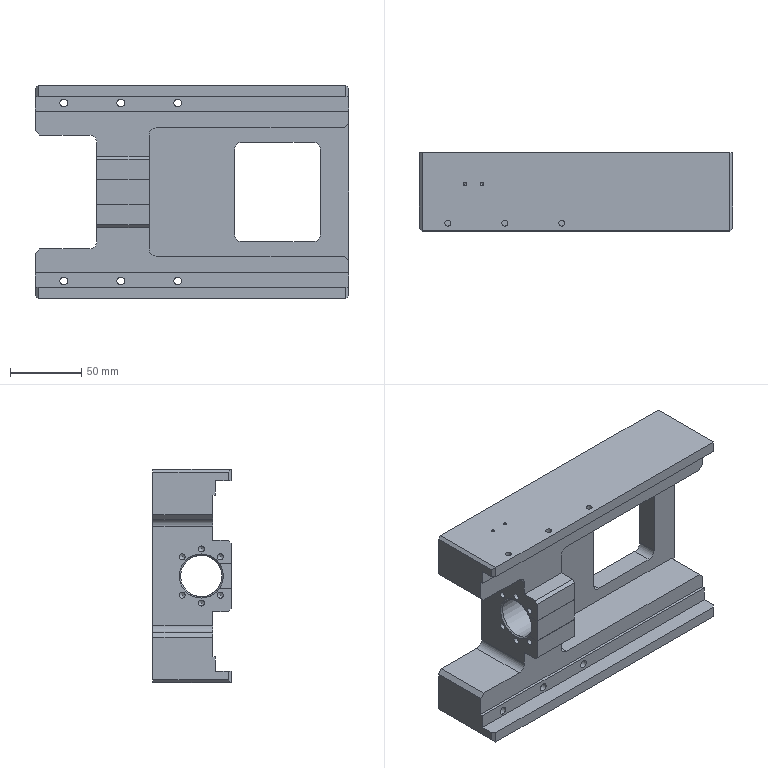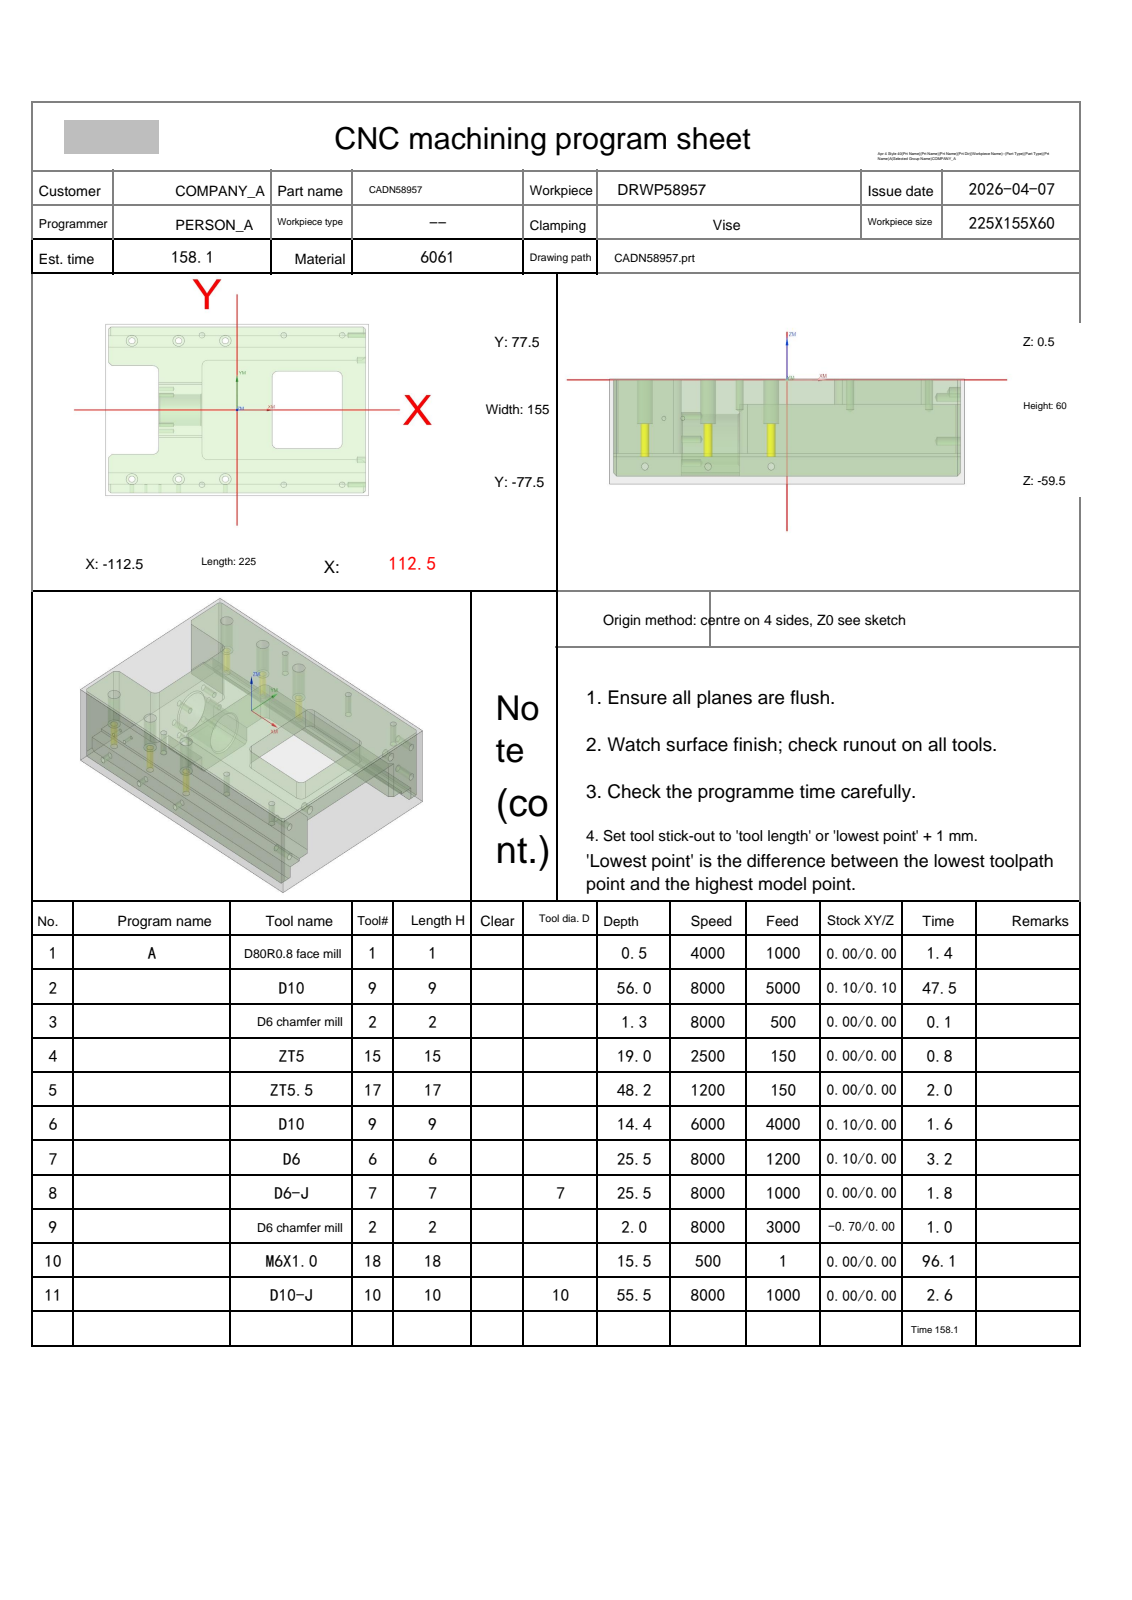NC program | NX | posted by the shop | part box 220 x 55 x 150 mm
Lines 11597 to 12878 of 12878:
N3 T02 M06
(D6 chamfer mill  D=6. R=0. H=02 ce=0.00 di=0.10)
G00 G90 G54 X90. Y67.5 M03 S8000
G43 H02 Z20.
M08
G98 G81 X90. Y67.5 Z-.8 R1. F500.
X40.
X-10. Y62.5
X-30. Y67.5
X-50. Y62.5
X-90.
Y-62.5
X-50.
X-30. Y-67.5
X-10. Y-62.5
X40. Y-67.5
X90.
G80
G00 Z20.
G91 G28 Z0.0
M05
M09
G91 G28 Z0.0
M01
N4 T15 M06
(ZT5 D=5. DR_a=118 H=15)
G00 G90 G54 X90. Y-67.5 M03 S2500
G43 H15 Z20.
M08
G98 G83 X90. Y-67.5 Z-18.502 R1. F150. Q3.
X40.
X-30.
Y67.5
X40.
X90.
G80
G00 Z20.
G91 G28 Z0.0
M05
M09
G91 G28 Z0.0
M01
N5 T17 M06
(ZT5.5 D=5.5 DR_a=118 H=17)
G00 G90 G54 X-90. Y-62.5 M03 S1200
G43 H17 Z20.
M08
G98 G83 X-90. Y-62.5 Z-47.652 R1. F150. Q2.
X-50.
X-10.
Y62.5
X-50.
X-90.
G80
G00 Z20.
G91 G28 Z0.0
M05
M09
G91 G28 Z0.0
M01
N6 T09 M06
(D10  D=10. R=0. H=09 ce=0.10 di=0.00)
G00 G90 G54 X84.9 Y0.0 M03 S6000
G43 H09 Z20.
M08
Z.5
G01 Y29.9 Z.432 F4000.
X35.1 Z.319
Y-29.9 Z.184
X84.9 Z.071
Y29.9 Z-.064
X35.1 Z-.177
Y-29.9 Z-.313
X84.9 Z-.425
Y29.9 Z-.561
X35.1 Z-.674
Y-29.9 Z-.809
X84.9 Z-.922
Y29.9 Z-1.057
X35.1 Z-1.17
Y-29.9 Z-1.306
X84.9 Z-1.418
Y29.9 Z-1.554
X35.1 Z-1.667
Y-29.9 Z-1.802
X84.9 Z-1.915
Y29.9 Z-2.05
X35.1 Z-2.163
Y-29.9 Z-2.299
X84.9 Z-2.412
Y29.9 Z-2.547
X35.1 Z-2.66
Y-29.9 Z-2.795
X84.9 Z-2.908
Y29.9 Z-3.044
X35.1 Z-3.156
Y-29.9 Z-3.292
X84.9 Z-3.405
Y29.9 Z-3.54
X35.1 Z-3.653
Y-29.9 Z-3.788
X84.9 Z-3.901
Y29.9 Z-4.037
X35.1 Z-4.15
Y-29.9 Z-4.285
X84.9 Z-4.398
Y29.9 Z-4.533
X35.1 Z-4.646
Y-29.9 Z-4.782
X84.9 Z-4.894
Y29.9 Z-5.03
X35.1 Z-5.143
Y-29.9 Z-5.278
X84.9 Z-5.391
Y29.9 Z-5.526
X35.1 Z-5.639
Y-29.9 Z-5.775
X84.9 Z-5.887
Y29.9 Z-6.023
X35.1 Z-6.136
Y-29.9 Z-6.271
X84.9 Z-6.384
Y29.9 Z-6.519
X35.1 Z-6.632
Y-29.9 Z-6.768
X84.9 Z-6.881
Y29.9 Z-7.016
X35.1 Z-7.129
Y-29.9 Z-7.264
X84.9 Z-7.377
Y29.9 Z-7.513
X35.1 Z-7.625
Y-29.9 Z-7.761
X84.9 Z-7.874
Y29.9 Z-8.009
X35.1 Z-8.122
Y-29.9 Z-8.257
X84.9 Z-8.37
Y29.9 Z-8.506
X35.1 Z-8.618
Y-29.9 Z-8.754
X84.9 Z-8.867
Y29.9 Z-9.002
X35.1 Z-9.115
Y-29.9 Z-9.25
X84.9 Z-9.363
Y29.9 Z-9.499
X35.1 Z-9.612
Y-29.9 Z-9.747
X84.9 Z-9.86
Y29.9 Z-9.995
X35.1 Z-10.108
Y-29.9 Z-10.244
X84.9 Z-10.356
Y29.9 Z-10.492
X35.1 Z-10.605
Y-29.9 Z-10.74
X84.9 Z-10.853
Y29.9 Z-10.988
X35.1 Z-11.101
Y-29.9 Z-11.237
X84.9 Z-11.35
Y29.9 Z-11.485
X35.1 Z-11.598
Y-29.9 Z-11.733
X84.9 Z-11.846
Y29.9 Z-11.982
X35.1 Z-12.094
Y-29.9 Z-12.23
X84.9 Z-12.343
Y29.9 Z-12.478
X35.1 Z-12.591
Y-29.9 Z-12.726
X84.9 Z-12.839
Y29.9 Z-12.975
X35.1 Z-13.087
Y-29.9 Z-13.223
X84.9 Z-13.336
Y29.9 Z-13.471
X35.1 Z-13.584
Y-29.9 Z-13.719
X84.9 Z-13.832
Y0.0 Z-13.9
Y29.9
X35.1
Y-29.9
X84.9
Y0.0
Y.5
Z-12.9
G00 Z20.
G91 G28 Z0.0
M05
M09
G91 G28 Z0.0
M01
N7 T06 M06
(D6  D=6. R=0. H=06 ce=0.10 di=0.00)
G00 G90 G54 X-90. Y-62.5 M03 S8000
G43 H06 Z20.
M08
Z.5
G03 X-89.05 Y-63.45 I.95 J0.0 F1200.
X-88.1 Y-62.5 I0.0 J.95
X-88.1 Y-62.5 Z0.0 I-1.9 J0.0
X-88.1 Y-62.5 Z-.5 I-1.9 J0.0
X-88.1 Y-62.5 Z-1. I-1.9 J0.0
X-88.1 Y-62.5 Z-1.5 I-1.9 J0.0
X-88.1 Y-62.5 Z-2. I-1.9 J0.0
X-88.1 Y-62.5 Z-2.5 I-1.9 J0.0
X-88.1 Y-62.5 Z-3. I-1.9 J0.0
X-88.1 Y-62.5 Z-3.5 I-1.9 J0.0
X-88.1 Y-62.5 Z-4. I-1.9 J0.0
X-88.1 Y-62.5 Z-4.5 I-1.9 J0.0
X-88.1 Y-62.5 Z-5. I-1.9 J0.0
X-88.1 Y-62.5 Z-5.5 I-1.9 J0.0
X-88.1 Y-62.5 Z-6. I-1.9 J0.0
X-88.1 Y-62.5 Z-6.5 I-1.9 J0.0
X-88.1 Y-62.5 Z-7. I-1.9 J0.0
X-88.1 Y-62.5 Z-7.5 I-1.9 J0.0
X-88.1 Y-62.5 Z-8. I-1.9 J0.0
X-88.1 Y-62.5 Z-8.5 I-1.9 J0.0
X-88.1 Y-62.5 Z-9. I-1.9 J0.0
X-88.1 Y-62.5 Z-9.5 I-1.9 J0.0
X-88.1 Y-62.5 Z-10. I-1.9 J0.0
X-88.1 Y-62.5 Z-10.5 I-1.9 J0.0
X-88.1 Y-62.5 Z-11. I-1.9 J0.0
X-88.1 Y-62.5 Z-11.5 I-1.9 J0.0
X-88.1 Y-62.5 Z-12. I-1.9 J0.0
X-88.1 Y-62.5 Z-12.5 I-1.9 J0.0
X-88.1 Y-62.5 Z-13. I-1.9 J0.0
X-88.1 Y-62.5 Z-13.5 I-1.9 J0.0
X-88.1 Y-62.5 Z-14. I-1.9 J0.0
X-88.1 Y-62.5 Z-14.5 I-1.9 J0.0
X-88.1 Y-62.5 Z-15. I-1.9 J0.0
X-88.1 Y-62.5 Z-15.5 I-1.9 J0.0
X-88.1 Y-62.5 Z-16. I-1.9 J0.0
X-88.1 Y-62.5 Z-16.5 I-1.9 J0.0
X-88.1 Y-62.5 Z-17. I-1.9 J0.0
X-88.1 Y-62.5 Z-17.5 I-1.9 J0.0
X-88.1 Y-62.5 Z-18. I-1.9 J0.0
X-88.1 Y-62.5 Z-18.5 I-1.9 J0.0
X-88.1 Y-62.5 Z-19. I-1.9 J0.0
X-88.1 Y-62.5 Z-19.5 I-1.9 J0.0
X-88.1 Y-62.5 Z-20. I-1.9 J0.0
X-88.1 Y-62.5 Z-20.5 I-1.9 J0.0
X-88.1 Y-62.5 Z-21. I-1.9 J0.0
X-88.1 Y-62.5 Z-21.5 I-1.9 J0.0
X-88.1 Y-62.5 Z-22. I-1.9 J0.0
X-88.1 Y-62.5 Z-22.5 I-1.9 J0.0
X-88.1 Y-62.5 Z-23. I-1.9 J0.0
X-88.1 Y-62.5 Z-23.5 I-1.9 J0.0
X-88.1 Y-62.5 Z-24. I-1.9 J0.0
X-88.1 Y-62.5 Z-24.5 I-1.9 J0.0
X-88.1 Y-62.5 Z-25. I-1.9 J0.0
X-90. Y-60.6 I-1.9 J0.0
X-91.9 Y-62.5 I0.0 J-1.9
X-90. Y-64.4 I1.9 J0.0
X-88.1 Y-62.5 I0.0 J1.9
X-89.05 Y-61.55 I-.95 J0.0
X-90. Y-62.5 I0.0 J-.95
G00 Z20.
X-50.
Z.5
G03 X-49.05 Y-63.45 I.95 J0.0
X-48.1 Y-62.5 I0.0 J.95
X-48.1 Y-62.5 Z0.0 I-1.9 J0.0
X-48.1 Y-62.5 Z-.5 I-1.9 J0.0
X-48.1 Y-62.5 Z-1. I-1.9 J0.0
X-48.1 Y-62.5 Z-1.5 I-1.9 J0.0
X-48.1 Y-62.5 Z-2. I-1.9 J0.0
X-48.1 Y-62.5 Z-2.5 I-1.9 J0.0
X-48.1 Y-62.5 Z-3. I-1.9 J0.0
X-48.1 Y-62.5 Z-3.5 I-1.9 J0.0
X-48.1 Y-62.5 Z-4. I-1.9 J0.0
X-48.1 Y-62.5 Z-4.5 I-1.9 J0.0
X-48.1 Y-62.5 Z-5. I-1.9 J0.0
X-48.1 Y-62.5 Z-5.5 I-1.9 J0.0
X-48.1 Y-62.5 Z-6. I-1.9 J0.0
X-48.1 Y-62.5 Z-6.5 I-1.9 J0.0
X-48.1 Y-62.5 Z-7. I-1.9 J0.0
X-48.1 Y-62.5 Z-7.5 I-1.9 J0.0
X-48.1 Y-62.5 Z-8. I-1.9 J0.0
X-48.1 Y-62.5 Z-8.5 I-1.9 J0.0
X-48.1 Y-62.5 Z-9. I-1.9 J0.0
X-48.1 Y-62.5 Z-9.5 I-1.9 J0.0
X-48.1 Y-62.5 Z-10. I-1.9 J0.0
X-48.1 Y-62.5 Z-10.5 I-1.9 J0.0
X-48.1 Y-62.5 Z-11. I-1.9 J0.0
X-48.1 Y-62.5 Z-11.5 I-1.9 J0.0
X-48.1 Y-62.5 Z-12. I-1.9 J0.0
X-48.1 Y-62.5 Z-12.5 I-1.9 J0.0
X-48.1 Y-62.5 Z-13. I-1.9 J0.0
X-48.1 Y-62.5 Z-13.5 I-1.9 J0.0
X-48.1 Y-62.5 Z-14. I-1.9 J0.0
X-48.1 Y-62.5 Z-14.5 I-1.9 J0.0
X-48.1 Y-62.5 Z-15. I-1.9 J0.0
X-48.1 Y-62.5 Z-15.5 I-1.9 J0.0
X-48.1 Y-62.5 Z-16. I-1.9 J0.0
X-48.1 Y-62.5 Z-16.5 I-1.9 J0.0
X-48.1 Y-62.5 Z-17. I-1.9 J0.0
X-48.1 Y-62.5 Z-17.5 I-1.9 J0.0
X-48.1 Y-62.5 Z-18. I-1.9 J0.0
X-48.1 Y-62.5 Z-18.5 I-1.9 J0.0
X-48.1 Y-62.5 Z-19. I-1.9 J0.0
X-48.1 Y-62.5 Z-19.5 I-1.9 J0.0
X-48.1 Y-62.5 Z-20. I-1.9 J0.0
X-48.1 Y-62.5 Z-20.5 I-1.9 J0.0
X-48.1 Y-62.5 Z-21. I-1.9 J0.0
X-48.1 Y-62.5 Z-21.5 I-1.9 J0.0
X-48.1 Y-62.5 Z-22. I-1.9 J0.0
X-48.1 Y-62.5 Z-22.5 I-1.9 J0.0
X-48.1 Y-62.5 Z-23. I-1.9 J0.0
X-48.1 Y-62.5 Z-23.5 I-1.9 J0.0
X-48.1 Y-62.5 Z-24. I-1.9 J0.0
X-48.1 Y-62.5 Z-24.5 I-1.9 J0.0
X-48.1 Y-62.5 Z-25. I-1.9 J0.0
X-50. Y-60.6 I-1.9 J0.0
X-51.9 Y-62.5 I0.0 J-1.9
X-50. Y-64.4 I1.9 J0.0
X-48.1 Y-62.5 I0.0 J1.9
X-49.05 Y-61.55 I-.95 J0.0
X-50. Y-62.5 I0.0 J-.95
G00 Z20.
X-10.
Z.5
G03 X-9.05 Y-63.45 I.95 J0.0
X-8.1 Y-62.5 I0.0 J.95
X-8.1 Y-62.5 Z0.0 I-1.9 J0.0
X-8.1 Y-62.5 Z-.5 I-1.9 J0.0
X-8.1 Y-62.5 Z-1. I-1.9 J0.0
X-8.1 Y-62.5 Z-1.5 I-1.9 J0.0
X-8.1 Y-62.5 Z-2. I-1.9 J0.0
X-8.1 Y-62.5 Z-2.5 I-1.9 J0.0
X-8.1 Y-62.5 Z-3. I-1.9 J0.0
X-8.1 Y-62.5 Z-3.5 I-1.9 J0.0
X-8.1 Y-62.5 Z-4. I-1.9 J0.0
X-8.1 Y-62.5 Z-4.5 I-1.9 J0.0
X-8.1 Y-62.5 Z-5. I-1.9 J0.0
X-8.1 Y-62.5 Z-5.5 I-1.9 J0.0
X-8.1 Y-62.5 Z-6. I-1.9 J0.0
X-8.1 Y-62.5 Z-6.5 I-1.9 J0.0
X-8.1 Y-62.5 Z-7. I-1.9 J0.0
X-8.1 Y-62.5 Z-7.5 I-1.9 J0.0
X-8.1 Y-62.5 Z-8. I-1.9 J0.0
X-8.1 Y-62.5 Z-8.5 I-1.9 J0.0
X-8.1 Y-62.5 Z-9. I-1.9 J0.0
X-8.1 Y-62.5 Z-9.5 I-1.9 J0.0
X-8.1 Y-62.5 Z-10. I-1.9 J0.0
X-8.1 Y-62.5 Z-10.5 I-1.9 J0.0
X-8.1 Y-62.5 Z-11. I-1.9 J0.0
X-8.1 Y-62.5 Z-11.5 I-1.9 J0.0
X-8.1 Y-62.5 Z-12. I-1.9 J0.0
X-8.1 Y-62.5 Z-12.5 I-1.9 J0.0
X-8.1 Y-62.5 Z-13. I-1.9 J0.0
X-8.1 Y-62.5 Z-13.5 I-1.9 J0.0
X-8.1 Y-62.5 Z-14. I-1.9 J0.0
X-8.1 Y-62.5 Z-14.5 I-1.9 J0.0
X-8.1 Y-62.5 Z-15. I-1.9 J0.0
X-8.1 Y-62.5 Z-15.5 I-1.9 J0.0
X-8.1 Y-62.5 Z-16. I-1.9 J0.0
X-8.1 Y-62.5 Z-16.5 I-1.9 J0.0
X-8.1 Y-62.5 Z-17. I-1.9 J0.0
X-8.1 Y-62.5 Z-17.5 I-1.9 J0.0
X-8.1 Y-62.5 Z-18. I-1.9 J0.0
X-8.1 Y-62.5 Z-18.5 I-1.9 J0.0
X-8.1 Y-62.5 Z-19. I-1.9 J0.0
X-8.1 Y-62.5 Z-19.5 I-1.9 J0.0
X-8.1 Y-62.5 Z-20. I-1.9 J0.0
X-8.1 Y-62.5 Z-20.5 I-1.9 J0.0
X-8.1 Y-62.5 Z-21. I-1.9 J0.0
X-8.1 Y-62.5 Z-21.5 I-1.9 J0.0
X-8.1 Y-62.5 Z-22. I-1.9 J0.0
X-8.1 Y-62.5 Z-22.5 I-1.9 J0.0
X-8.1 Y-62.5 Z-23. I-1.9 J0.0
X-8.1 Y-62.5 Z-23.5 I-1.9 J0.0
X-8.1 Y-62.5 Z-24. I-1.9 J0.0
X-8.1 Y-62.5 Z-24.5 I-1.9 J0.0
X-8.1 Y-62.5 Z-25. I-1.9 J0.0
X-10. Y-60.6 I-1.9 J0.0
X-11.9 Y-62.5 I0.0 J-1.9
X-10. Y-64.4 I1.9 J0.0
X-8.1 Y-62.5 I0.0 J1.9
X-9.05 Y-61.55 I-.95 J0.0
X-10. Y-62.5 I0.0 J-.95
G00 Z20.
Y62.5
Z.5
G03 X-9.05 Y61.55 I.95 J0.0
X-8.1 Y62.5 I0.0 J.95
X-8.1 Y62.5 Z0.0 I-1.9 J0.0
X-8.1 Y62.5 Z-.5 I-1.9 J0.0
X-8.1 Y62.5 Z-1. I-1.9 J0.0
X-8.1 Y62.5 Z-1.5 I-1.9 J0.0
X-8.1 Y62.5 Z-2. I-1.9 J0.0
X-8.1 Y62.5 Z-2.5 I-1.9 J0.0
X-8.1 Y62.5 Z-3. I-1.9 J0.0
X-8.1 Y62.5 Z-3.5 I-1.9 J0.0
X-8.1 Y62.5 Z-4. I-1.9 J0.0
X-8.1 Y62.5 Z-4.5 I-1.9 J0.0
X-8.1 Y62.5 Z-5. I-1.9 J0.0
X-8.1 Y62.5 Z-5.5 I-1.9 J0.0
X-8.1 Y62.5 Z-6. I-1.9 J0.0
X-8.1 Y62.5 Z-6.5 I-1.9 J0.0
X-8.1 Y62.5 Z-7. I-1.9 J0.0
X-8.1 Y62.5 Z-7.5 I-1.9 J0.0
X-8.1 Y62.5 Z-8. I-1.9 J0.0
X-8.1 Y62.5 Z-8.5 I-1.9 J0.0
X-8.1 Y62.5 Z-9. I-1.9 J0.0
X-8.1 Y62.5 Z-9.5 I-1.9 J0.0
X-8.1 Y62.5 Z-10. I-1.9 J0.0
X-8.1 Y62.5 Z-10.5 I-1.9 J0.0
X-8.1 Y62.5 Z-11. I-1.9 J0.0
X-8.1 Y62.5 Z-11.5 I-1.9 J0.0
X-8.1 Y62.5 Z-12. I-1.9 J0.0
X-8.1 Y62.5 Z-12.5 I-1.9 J0.0
X-8.1 Y62.5 Z-13. I-1.9 J0.0
X-8.1 Y62.5 Z-13.5 I-1.9 J0.0
X-8.1 Y62.5 Z-14. I-1.9 J0.0
X-8.1 Y62.5 Z-14.5 I-1.9 J0.0
X-8.1 Y62.5 Z-15. I-1.9 J0.0
X-8.1 Y62.5 Z-15.5 I-1.9 J0.0
X-8.1 Y62.5 Z-16. I-1.9 J0.0
X-8.1 Y62.5 Z-16.5 I-1.9 J0.0
X-8.1 Y62.5 Z-17. I-1.9 J0.0
X-8.1 Y62.5 Z-17.5 I-1.9 J0.0
X-8.1 Y62.5 Z-18. I-1.9 J0.0
X-8.1 Y62.5 Z-18.5 I-1.9 J0.0
X-8.1 Y62.5 Z-19. I-1.9 J0.0
X-8.1 Y62.5 Z-19.5 I-1.9 J0.0
X-8.1 Y62.5 Z-20. I-1.9 J0.0
X-8.1 Y62.5 Z-20.5 I-1.9 J0.0
X-8.1 Y62.5 Z-21. I-1.9 J0.0
X-8.1 Y62.5 Z-21.5 I-1.9 J0.0
X-8.1 Y62.5 Z-22. I-1.9 J0.0
X-8.1 Y62.5 Z-22.5 I-1.9 J0.0
X-8.1 Y62.5 Z-23. I-1.9 J0.0
X-8.1 Y62.5 Z-23.5 I-1.9 J0.0
X-8.1 Y62.5 Z-24. I-1.9 J0.0
X-8.1 Y62.5 Z-24.5 I-1.9 J0.0
X-8.1 Y62.5 Z-25. I-1.9 J0.0
X-10. Y64.4 I-1.9 J0.0
X-11.9 Y62.5 I0.0 J-1.9
X-10. Y60.6 I1.9 J0.0
X-8.1 Y62.5 I0.0 J1.9
X-9.05 Y63.45 I-.95 J0.0
X-10. Y62.5 I0.0 J-.95
G00 Z20.
X-50.
Z.5
G03 X-49.05 Y61.55 I.95 J0.0
X-48.1 Y62.5 I0.0 J.95
X-48.1 Y62.5 Z0.0 I-1.9 J0.0
X-48.1 Y62.5 Z-.5 I-1.9 J0.0
X-48.1 Y62.5 Z-1. I-1.9 J0.0
X-48.1 Y62.5 Z-1.5 I-1.9 J0.0
X-48.1 Y62.5 Z-2. I-1.9 J0.0
X-48.1 Y62.5 Z-2.5 I-1.9 J0.0
X-48.1 Y62.5 Z-3. I-1.9 J0.0
X-48.1 Y62.5 Z-3.5 I-1.9 J0.0
X-48.1 Y62.5 Z-4. I-1.9 J0.0
X-48.1 Y62.5 Z-4.5 I-1.9 J0.0
X-48.1 Y62.5 Z-5. I-1.9 J0.0
X-48.1 Y62.5 Z-5.5 I-1.9 J0.0
X-48.1 Y62.5 Z-6. I-1.9 J0.0
X-48.1 Y62.5 Z-6.5 I-1.9 J0.0
X-48.1 Y62.5 Z-7. I-1.9 J0.0
X-48.1 Y62.5 Z-7.5 I-1.9 J0.0
X-48.1 Y62.5 Z-8. I-1.9 J0.0
X-48.1 Y62.5 Z-8.5 I-1.9 J0.0
X-48.1 Y62.5 Z-9. I-1.9 J0.0
X-48.1 Y62.5 Z-9.5 I-1.9 J0.0
X-48.1 Y62.5 Z-10. I-1.9 J0.0
X-48.1 Y62.5 Z-10.5 I-1.9 J0.0
X-48.1 Y62.5 Z-11. I-1.9 J0.0
X-48.1 Y62.5 Z-11.5 I-1.9 J0.0
X-48.1 Y62.5 Z-12. I-1.9 J0.0
X-48.1 Y62.5 Z-12.5 I-1.9 J0.0
X-48.1 Y62.5 Z-13. I-1.9 J0.0
X-48.1 Y62.5 Z-13.5 I-1.9 J0.0
X-48.1 Y62.5 Z-14. I-1.9 J0.0
X-48.1 Y62.5 Z-14.5 I-1.9 J0.0
X-48.1 Y62.5 Z-15. I-1.9 J0.0
X-48.1 Y62.5 Z-15.5 I-1.9 J0.0
X-48.1 Y62.5 Z-16. I-1.9 J0.0
X-48.1 Y62.5 Z-16.5 I-1.9 J0.0
X-48.1 Y62.5 Z-17. I-1.9 J0.0
X-48.1 Y62.5 Z-17.5 I-1.9 J0.0
X-48.1 Y62.5 Z-18. I-1.9 J0.0
X-48.1 Y62.5 Z-18.5 I-1.9 J0.0
X-48.1 Y62.5 Z-19. I-1.9 J0.0
X-48.1 Y62.5 Z-19.5 I-1.9 J0.0
X-48.1 Y62.5 Z-20. I-1.9 J0.0
X-48.1 Y62.5 Z-20.5 I-1.9 J0.0
X-48.1 Y62.5 Z-21. I-1.9 J0.0
X-48.1 Y62.5 Z-21.5 I-1.9 J0.0
X-48.1 Y62.5 Z-22. I-1.9 J0.0
X-48.1 Y62.5 Z-22.5 I-1.9 J0.0
X-48.1 Y62.5 Z-23. I-1.9 J0.0
X-48.1 Y62.5 Z-23.5 I-1.9 J0.0
X-48.1 Y62.5 Z-24. I-1.9 J0.0
X-48.1 Y62.5 Z-24.5 I-1.9 J0.0
X-48.1 Y62.5 Z-25. I-1.9 J0.0
X-50. Y64.4 I-1.9 J0.0
X-51.9 Y62.5 I0.0 J-1.9
X-50. Y60.6 I1.9 J0.0
X-48.1 Y62.5 I0.0 J1.9
X-49.05 Y63.45 I-.95 J0.0
X-50. Y62.5 I0.0 J-.95
G00 Z20.
X-90.
Z.5
G03 X-89.05 Y61.55 I.95 J0.0
X-88.1 Y62.5 I0.0 J.95
X-88.1 Y62.5 Z0.0 I-1.9 J0.0
X-88.1 Y62.5 Z-.5 I-1.9 J0.0
X-88.1 Y62.5 Z-1. I-1.9 J0.0
X-88.1 Y62.5 Z-1.5 I-1.9 J0.0
X-88.1 Y62.5 Z-2. I-1.9 J0.0
X-88.1 Y62.5 Z-2.5 I-1.9 J0.0
X-88.1 Y62.5 Z-3. I-1.9 J0.0
X-88.1 Y62.5 Z-3.5 I-1.9 J0.0
X-88.1 Y62.5 Z-4. I-1.9 J0.0
X-88.1 Y62.5 Z-4.5 I-1.9 J0.0
X-88.1 Y62.5 Z-5. I-1.9 J0.0
X-88.1 Y62.5 Z-5.5 I-1.9 J0.0
X-88.1 Y62.5 Z-6. I-1.9 J0.0
X-88.1 Y62.5 Z-6.5 I-1.9 J0.0
X-88.1 Y62.5 Z-7. I-1.9 J0.0
X-88.1 Y62.5 Z-7.5 I-1.9 J0.0
X-88.1 Y62.5 Z-8. I-1.9 J0.0
X-88.1 Y62.5 Z-8.5 I-1.9 J0.0
X-88.1 Y62.5 Z-9. I-1.9 J0.0
X-88.1 Y62.5 Z-9.5 I-1.9 J0.0
X-88.1 Y62.5 Z-10. I-1.9 J0.0
X-88.1 Y62.5 Z-10.5 I-1.9 J0.0
X-88.1 Y62.5 Z-11. I-1.9 J0.0
X-88.1 Y62.5 Z-11.5 I-1.9 J0.0
X-88.1 Y62.5 Z-12. I-1.9 J0.0
X-88.1 Y62.5 Z-12.5 I-1.9 J0.0
X-88.1 Y62.5 Z-13. I-1.9 J0.0
X-88.1 Y62.5 Z-13.5 I-1.9 J0.0
X-88.1 Y62.5 Z-14. I-1.9 J0.0
X-88.1 Y62.5 Z-14.5 I-1.9 J0.0
X-88.1 Y62.5 Z-15. I-1.9 J0.0
X-88.1 Y62.5 Z-15.5 I-1.9 J0.0
X-88.1 Y62.5 Z-16. I-1.9 J0.0
X-88.1 Y62.5 Z-16.5 I-1.9 J0.0
X-88.1 Y62.5 Z-17. I-1.9 J0.0
X-88.1 Y62.5 Z-17.5 I-1.9 J0.0
X-88.1 Y62.5 Z-18. I-1.9 J0.0
X-88.1 Y62.5 Z-18.5 I-1.9 J0.0
X-88.1 Y62.5 Z-19. I-1.9 J0.0
X-88.1 Y62.5 Z-19.5 I-1.9 J0.0
X-88.1 Y62.5 Z-20. I-1.9 J0.0
X-88.1 Y62.5 Z-20.5 I-1.9 J0.0
X-88.1 Y62.5 Z-21. I-1.9 J0.0
X-88.1 Y62.5 Z-21.5 I-1.9 J0.0
X-88.1 Y62.5 Z-22. I-1.9 J0.0
X-88.1 Y62.5 Z-22.5 I-1.9 J0.0
X-88.1 Y62.5 Z-23. I-1.9 J0.0
X-88.1 Y62.5 Z-23.5 I-1.9 J0.0
X-88.1 Y62.5 Z-24. I-1.9 J0.0
X-88.1 Y62.5 Z-24.5 I-1.9 J0.0
X-88.1 Y62.5 Z-25. I-1.9 J0.0
X-90. Y64.4 I-1.9 J0.0
X-91.9 Y62.5 I0.0 J-1.9
X-90. Y60.6 I1.9 J0.0
X-88.1 Y62.5 I0.0 J1.9
X-89.05 Y63.45 I-.95 J0.0
X-90. Y62.5 I0.0 J-.95
G00 Z20.
G91 G28 Z0.0
M05
M09
G91 G28 Z0.0
M01
N8 T07 M06
(D6-J  D=6. R=0. H=07 ce=0.00 di=0.00)
G00 G90 G54 X-90. Y-62.5 M03 S8000
G43 H07 Z20.
M08
Z0.0
G41 D07
G01 X-89.96 Y-62.696 F500.
G03 X-88.99 Y-63.49 I.97 J.196
X-88. Y-62.5 I0.0 J.99
X-88. Y-62.5 Z-5. I-2. J0.0
X-88. Y-62.5 Z-10. I-2. J0.0
X-88. Y-62.5 Z-15. I-2. J0.0
X-88. Y-62.5 Z-20. I-2. J0.0
X-88. Y-62.5 Z-25. I-2. J0.0
X-90. Y-60.5 I-2. J0.0
X-92. Y-62.5 I0.0 J-2.
X-90. Y-64.5 I2. J0.0
X-88. Y-62.5 I0.0 J2.
X-88.99 Y-61.51 I-.99 J0.0
X-89.96 Y-62.304 I0.0 J-.99
G01 G40 X-90. Y-62.5
G00 Z20.
X-50.
Z0.0
G41 D07
G01 X-49.96 Y-62.696
G03 X-48.99 Y-63.49 I.97 J.196
X-48. Y-62.5 I0.0 J.99
X-48. Y-62.5 Z-5. I-2. J0.0
X-48. Y-62.5 Z-10. I-2. J0.0
X-48. Y-62.5 Z-15. I-2. J0.0
X-48. Y-62.5 Z-20. I-2. J0.0
X-48. Y-62.5 Z-25. I-2. J0.0
X-50. Y-60.5 I-2. J0.0
X-52. Y-62.5 I0.0 J-2.
X-50. Y-64.5 I2. J0.0
X-48. Y-62.5 I0.0 J2.
X-48.99 Y-61.51 I-.99 J0.0
X-49.96 Y-62.304 I0.0 J-.99
G01 G40 X-50. Y-62.5
G00 Z20.
X-10.
Z0.0
G41 D07
G01 X-9.96 Y-62.696
G03 X-8.99 Y-63.49 I.97 J.196
X-8. Y-62.5 I0.0 J.99
X-8. Y-62.5 Z-5. I-2. J0.0
X-8. Y-62.5 Z-10. I-2. J0.0
X-8. Y-62.5 Z-15. I-2. J0.0
X-8. Y-62.5 Z-20. I-2. J0.0
X-8. Y-62.5 Z-25. I-2. J0.0
X-10. Y-60.5 I-2. J0.0
X-12. Y-62.5 I0.0 J-2.
X-10. Y-64.5 I2. J0.0
X-8. Y-62.5 I0.0 J2.
X-8.99 Y-61.51 I-.99 J0.0
X-9.96 Y-62.304 I0.0 J-.99
G01 G40 X-10. Y-62.5
G00 Z20.
Y62.5
Z0.0
G41 D07
G01 X-9.96 Y62.304
G03 X-8.99 Y61.51 I.97 J.196
X-8. Y62.5 I0.0 J.99
X-8. Y62.5 Z-5. I-2. J0.0
X-8. Y62.5 Z-10. I-2. J0.0
X-8. Y62.5 Z-15. I-2. J0.0
X-8. Y62.5 Z-20. I-2. J0.0
X-8. Y62.5 Z-25. I-2. J0.0
X-10. Y64.5 I-2. J0.0
X-12. Y62.5 I0.0 J-2.
X-10. Y60.5 I2. J0.0
X-8. Y62.5 I0.0 J2.
X-8.99 Y63.49 I-.99 J0.0
X-9.96 Y62.696 I0.0 J-.99
G01 G40 X-10. Y62.5
G00 Z20.
X-50.
Z0.0
G41 D07
G01 X-49.96 Y62.304
G03 X-48.99 Y61.51 I.97 J.196
X-48. Y62.5 I0.0 J.99
X-48. Y62.5 Z-5. I-2. J0.0
X-48. Y62.5 Z-10. I-2. J0.0
X-48. Y62.5 Z-15. I-2. J0.0
X-48. Y62.5 Z-20. I-2. J0.0
X-48. Y62.5 Z-25. I-2. J0.0
X-50. Y64.5 I-2. J0.0
X-52. Y62.5 I0.0 J-2.
X-50. Y60.5 I2. J0.0
X-48. Y62.5 I0.0 J2.
X-48.99 Y63.49 I-.99 J0.0
X-49.96 Y62.696 I0.0 J-.99
G01 G40 X-50. Y62.5
G00 Z20.
X-90.
Z0.0
G41 D07
G01 X-89.96 Y62.304
G03 X-88.99 Y61.51 I.97 J.196
X-88. Y62.5 I0.0 J.99
X-88. Y62.5 Z-5. I-2. J0.0
X-88. Y62.5 Z-10. I-2. J0.0
X-88. Y62.5 Z-15. I-2. J0.0
X-88. Y62.5 Z-20. I-2. J0.0
X-88. Y62.5 Z-25. I-2. J0.0
X-90. Y64.5 I-2. J0.0
X-92. Y62.5 I0.0 J-2.
X-90. Y60.5 I2. J0.0
X-88. Y62.5 I0.0 J2.
X-88.99 Y63.49 I-.99 J0.0
X-89.96 Y62.696 I0.0 J-.99
G01 G40 X-90. Y62.5
G00 Z20.
G00 G90 X84.801 Y-31. M03 S6000
Z20.
Z-6.25
G01 Z-6.75 F1000.
G41 D07
X86.
G03 X87. Y-30. I0.0 J1.
G01 Y30.
G03 X85. Y32. I-2. J0.0
G01 X35.
G03 X33. Y30. I0.0 J-2.
G01 Y-30.
G03 X35. Y-32. I2. J0.0
G01 X85.
G03 X87. Y-30. I0.0 J2.
G01 Y-29.5
G03 X86. Y-28.5 I-1. J0.0
G01 G40 X85.8
Z-6.25
G00 X84.801 Y-31.
Z-13.
G01 Z-13.5
G41 D07
X86.
G03 X87. Y-30. I0.0 J1.
G01 Y30.
G03 X85. Y32. I-2. J0.0
G01 X35.
G03 X33. Y30. I0.0 J-2.
G01 Y-30.
G03 X35. Y-32. I2. J0.0
G01 X85.
G03 X87. Y-30. I0.0 J2.
G01 Y-29.5
G03 X86. Y-28.5 I-1. J0.0
G01 G40 X85.8
Z-13.
G00 Z20.
G00 G90 X84.901 Y-31. M03 S6000
Z20.
Z-13.4
G01 Z-13.9 F1000.
G41 D07
X86.
G03 X87. Y-30. I0.0 J1.
G01 Y30.
G03 X85. Y32. I-2. J0.0
G01 X35.
G03 X33. Y30. I0.0 J-2.
G01 Y-30.
G03 X35. Y-32. I2. J0.0
G01 X85.
G03 X87. Y-30. I0.0 J2.
G01 Y-29.5
G03 X86. Y-28.5 I-1. J0.0
G01 G40 X85.9
Z-13.4
G00 Z20.
G91 G28 Z0.0
M05
M09
G91 G28 Z0.0
M01
N9 T02 M06
(D6 chamfer mill  D=6. R=0. H=02 ce=0.00 di=0.00)
G00 G90 G54 X.25 Y-77.128 M03 S8000
G43 H02 Z20.
M08
Z2.099
G01 Z-1.5 F3000.
G03 X.33 Y-76.828 I-.52 J.3
X.03 Y-76.308 I-.6 J0.0
G01 X0.0 Y-76.3
X-108.
X-108.254 Y-76.275
X-108.497 Y-76.201
X-108.722 Y-76.081
X-108.919 Y-75.919
X-110.919 Y-73.919
X-111.081 Y-73.722
X-111.201 Y-73.497
X-111.275 Y-73.254
X-111.3 Y-73.
Y-43.
X-111.275 Y-42.746
X-111.201 Y-42.503
X-111.081 Y-42.278
X-110.919 Y-42.081
X-107.919 Y-39.081
X-107.722 Y-38.919
X-107.497 Y-38.799
X-107.254 Y-38.725
X-107. Y-38.7
X-72.
G03 X-68.3 Y-35. I0.0 J3.7
G01 Y35.
G03 X-72. Y38.7 I-3.7 J0.0
G01 X-107.
X-107.254 Y38.725
X-107.497 Y38.799
X-107.722 Y38.919
X-107.919 Y39.081
X-110.919 Y42.081
X-111.081 Y42.278
X-111.201 Y42.503
X-111.275 Y42.746
X-111.3 Y43.
Y73.
X-111.275 Y73.254
X-111.201 Y73.497
X-111.081 Y73.722
X-110.919 Y73.919
X-108.919 Y75.919
X-108.722 Y76.081
X-108.497 Y76.201
X-108.254 Y76.275
X-108. Y76.3
X108.
X108.254 Y76.275
X108.497 Y76.201
X108.722 Y76.081
X108.919 Y75.919
X110.919 Y73.919
X111.081 Y73.722
X111.201 Y73.497
X111.275 Y73.254
X111.3 Y73.
Y-73.
X111.275 Y-73.254
X111.201 Y-73.497
X111.081 Y-73.722
X110.919 Y-73.919
X108.919 Y-75.919
X108.722 Y-76.081
X108.497 Y-76.201
X108.254 Y-76.275
X108. Y-76.3
X0.0
X-.03 Y-76.308
G03 X-.33 Y-76.828 I.3 J-.52
X-.25 Y-77.128 I.6 J0.0
G01 Z2.099
G00 Z20.
X32.128 Y.25
Z2.099
G01 Z-1.5
G03 X31.828 Y.33 I-.3 J-.52
X31.308 Y.03 I0.0 J-.6
G01 X31.3 Y0.0
Y-30.
G03 X35. Y-33.7 I3.7 J0.0
G01 X85.
G03 X88.7 Y-30. I0.0 J3.7
G01 Y30.
G03 X85. Y33.7 I-3.7 J0.0
G01 X35.
G03 X31.3 Y30. I0.0 J-3.7
G01 Y0.0
X31.308 Y-.03
G03 X31.828 Y-.33 I.52 J.3
X32.128 Y-.25 I0.0 J.6
G01 Z2.099
G00 Z20.
G00 G90 X-30.87 Y67.268 M03 S8000
Z20.
Z-.8
G01 Z-1.3 F600.
X-31.5 Y67.1
G03 X-30. Y65.6 I1.5 J0.0
X-28.1 Y67.5 I0.0 J1.9
X-30. Y69.4 I-1.9 J0.0
X-31.9 Y67.5 I0.0 J-1.9
X-30. Y65.6 I1.9 J0.0
X-28.5 Y67.1 I0.0 J1.5
G01 X-29.13 Y67.268
Z-.8
G00 Z20.
X39.13
Z-.8
G01 Z-1.3
X38.5 Y67.1
G03 X40. Y65.6 I1.5 J0.0
X41.9 Y67.5 I0.0 J1.9
X40. Y69.4 I-1.9 J0.0
X38.1 Y67.5 I0.0 J-1.9
X40. Y65.6 I1.9 J0.0
X41.5 Y67.1 I0.0 J1.5
G01 X40.87 Y67.268
Z-.8
G00 Z20.
X89.13
Z-.8
G01 Z-1.3
X88.5 Y67.1
G03 X90. Y65.6 I1.5 J0.0
X91.9 Y67.5 I0.0 J1.9
X90. Y69.4 I-1.9 J0.0
X88.1 Y67.5 I0.0 J-1.9
X90. Y65.6 I1.9 J0.0
X91.5 Y67.1 I0.0 J1.5
G01 X90.87 Y67.268
Z-.8
G00 Z20.
X89.13 Y-67.732
Z-.8
G01 Z-1.3
X88.5 Y-67.9
G03 X90. Y-69.4 I1.5 J0.0
X91.9 Y-67.5 I0.0 J1.9
X90. Y-65.6 I-1.9 J0.0
X88.1 Y-67.5 I0.0 J-1.9
X90. Y-69.4 I1.9 J0.0
X91.5 Y-67.9 I0.0 J1.5
G01 X90.87 Y-67.732
Z-.8
G00 Z20.
X39.13
Z-.8
G01 Z-1.3
X38.5 Y-67.9
G03 X40. Y-69.4 I1.5 J0.0
X41.9 Y-67.5 I0.0 J1.9
X40. Y-65.6 I-1.9 J0.0
X38.1 Y-67.5 I0.0 J-1.9
X40. Y-69.4 I1.9 J0.0
X41.5 Y-67.9 I0.0 J1.5
G01 X40.87 Y-67.732
Z-.8
G00 Z20.
X-30.87
Z-.8
G01 Z-1.3
X-31.5 Y-67.9
G03 X-30. Y-69.4 I1.5 J0.0
X-28.1 Y-67.5 I0.0 J1.9
X-30. Y-65.6 I-1.9 J0.0
X-31.9 Y-67.5 I0.0 J-1.9
X-30. Y-69.4 I1.9 J0.0
X-28.5 Y-67.9 I0.0 J1.5
G01 X-29.13 Y-67.732
Z-.8
G00 Z20.
G00 G90 X-86.614 Y-65.154 M03 S8000
Z20.
Z2.5
G01 X-86.606 Y-65.145 Z2.495 F800.
X-86.356 Y-64.789 Z2.337
X-86.196 Y-64.511 Z2.22
X-86.012 Y-64.117 Z2.062
X-85.87 Y-63.707 Z1.904
X-85.769 Y-63.284 Z1.746
X-85.712 Y-62.854 Z1.588
X-85.698 Y-62.42 Z1.43
X-85.728 Y-61.986 Z1.272
X-85.801 Y-61.558 Z1.114
X-85.918 Y-61.14 Z.956
X-86.076 Y-60.735 Z.797
X-86.273 Y-60.349 Z.639
X-86.509 Y-59.984 Z.481
X-86.781 Y-59.645 Z.323
X-87.085 Y-59.335 Z.165
X-87.419 Y-59.057 Z.007
X-87.779 Y-58.814 Z-.151
X-88.162 Y-58.609 Z-.309
X-88.564 Y-58.444 Z-.467
X-88.98 Y-58.32 Z-.625
X-89.407 Y-58.238 Z-.783
X-89.839 Y-58.2 Z-.942
X-90. Z-1.
G03 X-94.3 Y-62.5 I0.0 J-4.3
X-90. Y-66.8 I4.3 J0.0
X-85.7 Y-62.5 I0.0 J4.3
X-90. Y-58.2 I-4.3 J0.0
X-90.499 Y-58.229 I0.0 J-4.3
G01 Z1.5
G00 Z20.
X-46.614 Y-65.154
Z2.5
G01 X-46.606 Y-65.145 Z2.495
X-46.356 Y-64.789 Z2.337
X-46.196 Y-64.511 Z2.22
X-46.012 Y-64.117 Z2.062
X-45.87 Y-63.707 Z1.904
X-45.769 Y-63.284 Z1.746
X-45.712 Y-62.854 Z1.588
X-45.698 Y-62.42 Z1.43
X-45.728 Y-61.986 Z1.272
X-45.801 Y-61.558 Z1.114
X-45.918 Y-61.14 Z.956
X-46.076 Y-60.735 Z.797
X-46.273 Y-60.349 Z.639
X-46.509 Y-59.984 Z.481
X-46.781 Y-59.645 Z.323
X-47.085 Y-59.335 Z.165
X-47.419 Y-59.057 Z.007
X-47.779 Y-58.814 Z-.151
X-48.162 Y-58.609 Z-.309
X-48.564 Y-58.444 Z-.467
X-48.98 Y-58.32 Z-.625
X-49.407 Y-58.238 Z-.783
X-49.839 Y-58.2 Z-.942
X-50. Z-1.
G03 X-54.3 Y-62.5 I0.0 J-4.3
X-50. Y-66.8 I4.3 J0.0
X-45.7 Y-62.5 I0.0 J4.3
X-50. Y-58.2 I-4.3 J0.0
X-50.499 Y-58.229 I0.0 J-4.3
G01 Z1.5
G00 Z20.
X-6.614 Y-65.154
Z2.5
G01 X-6.606 Y-65.145 Z2.495
X-6.356 Y-64.789 Z2.337
X-6.196 Y-64.511 Z2.22
X-6.012 Y-64.117 Z2.062
X-5.87 Y-63.707 Z1.904
X-5.769 Y-63.284 Z1.746
X-5.712 Y-62.854 Z1.588
X-5.698 Y-62.42 Z1.43
X-5.728 Y-61.986 Z1.272
X-5.801 Y-61.558 Z1.114
X-5.918 Y-61.14 Z.956
X-6.076 Y-60.735 Z.797
X-6.273 Y-60.349 Z.639
X-6.509 Y-59.984 Z.481
X-6.781 Y-59.645 Z.323
X-7.085 Y-59.335 Z.165
X-7.419 Y-59.057 Z.007
X-7.779 Y-58.814 Z-.151
X-8.162 Y-58.609 Z-.309
X-8.564 Y-58.444 Z-.467
X-8.98 Y-58.32 Z-.625
X-9.407 Y-58.238 Z-.783
X-9.839 Y-58.2 Z-.942
X-10. Z-1.
G03 X-14.3 Y-62.5 I0.0 J-4.3
X-10. Y-66.8 I4.3 J0.0
X-5.7 Y-62.5 I0.0 J4.3
X-10. Y-58.2 I-4.3 J0.0
X-10.499 Y-58.229 I0.0 J-4.3
G01 Z1.5
G00 Z20.
X-6.614 Y59.846
Z2.5
G01 X-6.606 Y59.855 Z2.495
X-6.356 Y60.211 Z2.337
X-6.196 Y60.489 Z2.22
X-6.012 Y60.883 Z2.062
X-5.87 Y61.293 Z1.904
X-5.769 Y61.716 Z1.746
X-5.712 Y62.146 Z1.588
X-5.698 Y62.58 Z1.43
X-5.728 Y63.014 Z1.272
X-5.801 Y63.442 Z1.114
X-5.918 Y63.86 Z.956
X-6.076 Y64.265 Z.797
X-6.273 Y64.652 Z.639
X-6.509 Y65.016 Z.481
X-6.781 Y65.355 Z.323
X-7.085 Y65.665 Z.165
X-7.419 Y65.943 Z.007
X-7.779 Y66.186 Z-.151
X-8.162 Y66.391 Z-.309
X-8.564 Y66.556 Z-.467
X-8.98 Y66.68 Z-.625
X-9.407 Y66.762 Z-.783
X-9.839 Y66.8 Z-.942
X-10. Z-1.
G03 X-14.3 Y62.5 I0.0 J-4.3
X-10. Y58.2 I4.3 J0.0
X-5.7 Y62.5 I0.0 J4.3
X-10. Y66.8 I-4.3 J0.0
X-10.499 Y66.771 I0.0 J-4.3
G01 Z1.5
G00 Z20.
X-46.614 Y59.846
Z2.5
G01 X-46.606 Y59.855 Z2.495
X-46.356 Y60.211 Z2.337
X-46.196 Y60.489 Z2.22
X-46.012 Y60.883 Z2.062
X-45.87 Y61.293 Z1.904
X-45.769 Y61.716 Z1.746
X-45.712 Y62.146 Z1.588
X-45.698 Y62.58 Z1.43
X-45.728 Y63.014 Z1.272
X-45.801 Y63.442 Z1.114
X-45.918 Y63.86 Z.956
X-46.076 Y64.265 Z.797
X-46.273 Y64.652 Z.639
X-46.509 Y65.016 Z.481
X-46.781 Y65.355 Z.323
X-47.085 Y65.665 Z.165
X-47.419 Y65.943 Z.007
X-47.779 Y66.186 Z-.151
X-48.162 Y66.391 Z-.309
X-48.564 Y66.556 Z-.467
X-48.98 Y66.68 Z-.625
X-49.407 Y66.762 Z-.783
X-49.839 Y66.8 Z-.942
X-50. Z-1.
G03 X-54.3 Y62.5 I0.0 J-4.3
X-50. Y58.2 I4.3 J0.0
X-45.7 Y62.5 I0.0 J4.3
X-50. Y66.8 I-4.3 J0.0
X-50.499 Y66.771 I0.0 J-4.3
G01 Z1.5
G00 Z20.
X-86.614 Y59.846
Z2.5
G01 X-86.606 Y59.855 Z2.495
X-86.356 Y60.211 Z2.337
X-86.196 Y60.489 Z2.22
X-86.012 Y60.883 Z2.062
X-85.87 Y61.293 Z1.904
X-85.769 Y61.716 Z1.746
X-85.712 Y62.146 Z1.588
X-85.698 Y62.58 Z1.43
X-85.728 Y63.014 Z1.272
X-85.801 Y63.442 Z1.114
X-85.918 Y63.86 Z.956
X-86.076 Y64.265 Z.797
X-86.273 Y64.652 Z.639
X-86.509 Y65.016 Z.481
X-86.781 Y65.355 Z.323
X-87.085 Y65.665 Z.165
X-87.419 Y65.943 Z.007
X-87.779 Y66.186 Z-.151
X-88.162 Y66.391 Z-.309
X-88.564 Y66.556 Z-.467
X-88.98 Y66.68 Z-.625
X-89.407 Y66.762 Z-.783
X-89.839 Y66.8 Z-.942
X-90. Z-1.
G03 X-94.3 Y62.5 I0.0 J-4.3
X-90. Y58.2 I4.3 J0.0
X-85.7 Y62.5 I0.0 J4.3
X-90. Y66.8 I-4.3 J0.0
X-90.499 Y66.771 I0.0 J-4.3
G01 Z1.5
G00 Z20.
G91 G28 Z0.0
M05
M09
G91 G28 Z0.0
M01
N10 T18 M06
(M6X1.0 D=5. DR_a=180 H=18)
G00 G90 G54 X90. Y-67.5 M03 S500
G43 H18 Z20.
M08
G95
G98 G84 X90. Y-67.5 Z-15. R1. F1. Q3.
X40.
X-30.
Y67.5
X40.
X90.
G80
G94
G00 Z20.
G91 G28 Z0.0
M05
M09
G91 G28 Z0.0
M01
N11 T10 M06
(D10-J  D=10. R=0. H=10 ce=0.00 di=0.00)
G00 G90 G54 X109.013 Y-81.116 M03 S8000
G43 H10 Z20.
M08
Z-17.833
G01 Z-18.333 F1000.
G41 D10
X108.997 Y-80.917
G03 X108. Y-80. I-.997 J-.083
G01 X-108.
G02 X-111.536 Y-78.536 I0.0 J5.
G01 X-113.536 Y-76.536
G02 X-115. Y-73. I3.536 J3.536
G01 Y-43.
G02 X-113.536 Y-39.464 I5. J0.0
G01 X-110.536 Y-36.464
G02 X-107. Y-35. I3.536 J-3.536
G01 X-72.
Y35.
X-107.
G02 X-110.536 Y36.464 I0.0 J5.
G01 X-113.536 Y39.464
G02 X-115. Y43. I3.536 J3.536
G01 Y73.
G02 X-113.536 Y76.536 I5. J0.0
G01 X-111.536 Y78.536
G02 X-108. Y80. I3.536 J-3.536
G01 X108.
G02 X111.536 Y78.536 I0.0 J-5.
G01 X113.536 Y76.536
G02 X115. Y73. I-3.536 J-3.536
G01 Y-73.
G02 X113.536 Y-76.536 I-5. J0.0
G01 X111.536 Y-78.536
G02 X108. Y-80. I-3.536 J3.536
G01 X107.5
G03 X106.5 Y-81. I0.0 J-1.
G01 G40 Y-81.2
Z-17.833
G00 Z20.
X109.013 Y-81.116
Z-36.167
G01 Z-36.667
G41 D10
X108.997 Y-80.917
G03 X108. Y-80. I-.997 J-.083
G01 X-108.
G02 X-111.536 Y-78.536 I0.0 J5.
G01 X-113.536 Y-76.536
G02 X-115. Y-73. I3.536 J3.536
G01 Y-43.
G02 X-113.536 Y-39.464 I5. J0.0
G01 X-110.536 Y-36.464
G02 X-107. Y-35. I3.536 J-3.536
G01 X-72.
Y35.
X-107.
G02 X-110.536 Y36.464 I0.0 J5.
G01 X-113.536 Y39.464
G02 X-115. Y43. I3.536 J3.536
G01 Y73.
G02 X-113.536 Y76.536 I5. J0.0
G01 X-111.536 Y78.536
G02 X-108. Y80. I3.536 J-3.536
G01 X108.
G02 X111.536 Y78.536 I0.0 J-5.
G01 X113.536 Y76.536
G02 X115. Y73. I-3.536 J-3.536
G01 Y-73.
G02 X113.536 Y-76.536 I-5. J0.0
G01 X111.536 Y-78.536
G02 X108. Y-80. I-3.536 J3.536
G01 X107.5
G03 X106.5 Y-81. I0.0 J-1.
G01 G40 Y-81.2
Z-36.167
G00 Z20.
X109.013 Y-81.116
Z-54.5
G01 Z-55.
G41 D10
X108.997 Y-80.917
G03 X108. Y-80. I-.997 J-.083
G01 X-108.
G02 X-111.536 Y-78.536 I0.0 J5.
G01 X-113.536 Y-76.536
G02 X-115. Y-73. I3.536 J3.536
G01 Y-43.
G02 X-113.536 Y-39.464 I5. J0.0
G01 X-110.536 Y-36.464
G02 X-107. Y-35. I3.536 J-3.536
G01 X-72.
Y35.
X-107.
G02 X-110.536 Y36.464 I0.0 J5.
G01 X-113.536 Y39.464
G02 X-115. Y43. I3.536 J3.536
G01 Y73.
G02 X-113.536 Y76.536 I5. J0.0
G01 X-111.536 Y78.536
G02 X-108. Y80. I3.536 J-3.536
G01 X108.
G02 X111.536 Y78.536 I0.0 J-5.
G01 X113.536 Y76.536
G02 X115. Y73. I-3.536 J-3.536
G01 Y-73.
G02 X113.536 Y-76.536 I-5. J0.0
G01 X111.536 Y-78.536
G02 X108. Y-80. I-3.536 J3.536
G01 X107.5
G03 X106.5 Y-81. I0.0 J-1.
G01 G40 Y-81.2
Z-54.5
G00 Z20.
M05
M09
G91 G28 Z0.0
G91 G28 Y0.0
M30
%